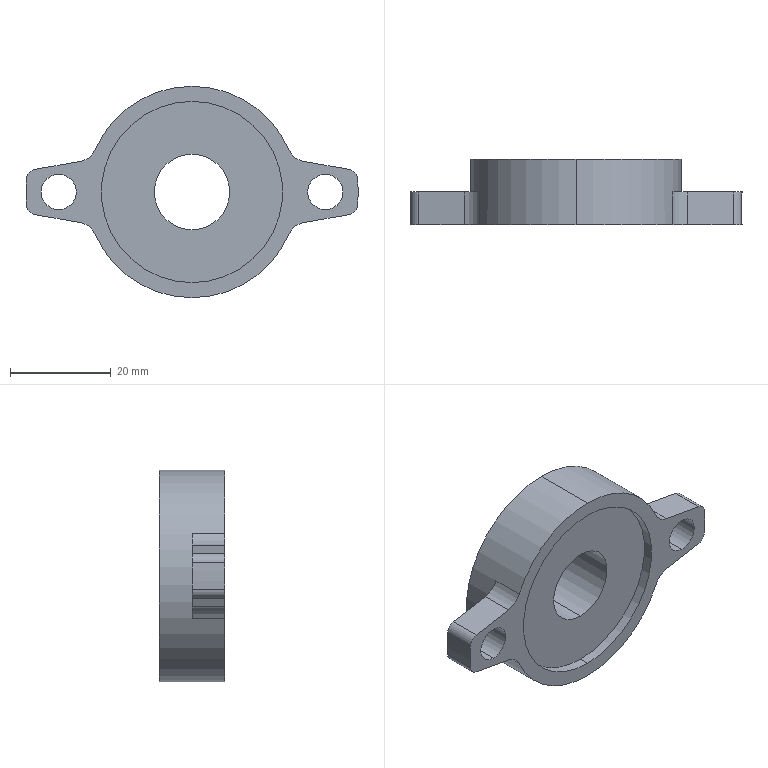Part | SolidWorks | features ICE 3, Fillet 2, Extrusion 1 | 1 solid | 29 faces | box 66 x 13 x 42 mm | volume 15219 mm3 | cylinder 20 | plane 9 | commonest cylinder face diameters 4 x4 7 x4 8 x4 15 x2 36 x2 42 x2
STEP:
#1=CARTESIAN_POINT('',(0.,2.,18.));
#2=VERTEX_POINT('',#1);
#3=CARTESIAN_POINT('',(0.,2.,-18.));
#4=VERTEX_POINT('',#3);
#5=CARTESIAN_POINT('',(0.,2.,0.));
#6=DIRECTION('',(0.,-1.,0.));
#7=DIRECTION('',(0.,0.,-1.));
#8=AXIS2_PLACEMENT_3D('',#5,#6,#7);
#9=CIRCLE('',#8,18.);
#10=EDGE_CURVE('',#2,#4,#9,.T.);
#11=ORIENTED_EDGE('',*,*,#10,.F.);
#12=CARTESIAN_POINT('',(0.,0.,18.));
#13=VERTEX_POINT('',#12);
#14=CARTESIAN_POINT('',(0.,2.,18.));
#15=DIRECTION('',(0.,-1.,0.));
#16=VECTOR('',#15,1000.);
#17=LINE('',#14,#16);
#18=EDGE_CURVE('',#2,#13,#17,.T.);
#19=ORIENTED_EDGE('',*,*,#18,.T.);
#20=CARTESIAN_POINT('',(0.,0.,-18.));
#21=VERTEX_POINT('',#20);
#22=CARTESIAN_POINT('',(0.,0.,0.));
#23=DIRECTION('',(0.,-1.,0.));
#24=DIRECTION('',(0.,0.,-1.));
#25=AXIS2_PLACEMENT_3D('',#22,#23,#24);
#26=CIRCLE('',#25,18.);
#27=EDGE_CURVE('',#13,#21,#26,.T.);
#28=ORIENTED_EDGE('',*,*,#27,.T.);
#29=CARTESIAN_POINT('',(0.,2.,-18.));
#30=DIRECTION('',(0.,-1.,0.));
#31=VECTOR('',#30,1000.);
#32=LINE('',#29,#31);
#33=EDGE_CURVE('',#4,#21,#32,.T.);
#34=ORIENTED_EDGE('',*,*,#33,.F.);
#35=EDGE_LOOP('',(#11,#19,#28,#34));
#36=FACE_OUTER_BOUND('',#35,.T.);
#37=CARTESIAN_POINT('',(0.,2.,0.));
#38=DIRECTION('',(0.,-1.,0.));
#39=DIRECTION('',(0.,0.,-1.));
#40=AXIS2_PLACEMENT_3D('',#37,#38,#39);
#41=CYLINDRICAL_SURFACE('',#40,18.);
#42=ADVANCED_FACE('',(#36),#41,.F.);
#43=CARTESIAN_POINT('',(26.5,0.,-3.5));
#44=VERTEX_POINT('',#43);
#45=CARTESIAN_POINT('',(26.5,0.,3.5));
#46=VERTEX_POINT('',#45);
#47=CARTESIAN_POINT('',(26.5,0.,0.));
#48=DIRECTION('',(0.,1.,0.));
#49=DIRECTION('',(0.,0.,1.));
#50=AXIS2_PLACEMENT_3D('',#47,#48,#49);
#51=CIRCLE('',#50,3.5);
#52=EDGE_CURVE('',#44,#46,#51,.T.);
#53=ORIENTED_EDGE('',*,*,#52,.F.);
#54=CARTESIAN_POINT('',(26.5,6.5,-3.5));
#55=VERTEX_POINT('',#54);
#56=CARTESIAN_POINT('',(26.5,0.,-3.5));
#57=DIRECTION('',(0.,1.,0.));
#58=VECTOR('',#57,1000.);
#59=LINE('',#56,#58);
#60=EDGE_CURVE('',#44,#55,#59,.T.);
#61=ORIENTED_EDGE('',*,*,#60,.T.);
#62=CARTESIAN_POINT('',(26.5,6.5,3.5));
#63=VERTEX_POINT('',#62);
#64=CARTESIAN_POINT('',(26.5,6.5,0.));
#65=DIRECTION('',(0.,1.,0.));
#66=DIRECTION('',(0.,0.,1.));
#67=AXIS2_PLACEMENT_3D('',#64,#65,#66);
#68=CIRCLE('',#67,3.5);
#69=EDGE_CURVE('',#55,#63,#68,.T.);
#70=ORIENTED_EDGE('',*,*,#69,.T.);
#71=CARTESIAN_POINT('',(26.5,0.,3.5));
#72=DIRECTION('',(0.,1.,0.));
#73=VECTOR('',#72,1000.);
#74=LINE('',#71,#73);
#75=EDGE_CURVE('',#46,#63,#74,.T.);
#76=ORIENTED_EDGE('',*,*,#75,.F.);
#77=EDGE_LOOP('',(#53,#61,#70,#76));
#78=FACE_OUTER_BOUND('',#77,.T.);
#79=CARTESIAN_POINT('',(26.5,0.,0.));
#80=DIRECTION('',(0.,1.,0.));
#81=DIRECTION('',(0.,0.,1.));
#82=AXIS2_PLACEMENT_3D('',#79,#80,#81);
#83=CYLINDRICAL_SURFACE('',#82,3.5);
#84=ADVANCED_FACE('',(#78),#83,.F.);
#85=CARTESIAN_POINT('',(-26.5,0.,-3.5));
#86=VERTEX_POINT('',#85);
#87=CARTESIAN_POINT('',(-26.5,0.,3.5));
#88=VERTEX_POINT('',#87);
#89=CARTESIAN_POINT('',(-26.5,0.,0.));
#90=DIRECTION('',(0.,1.,0.));
#91=DIRECTION('',(0.,0.,1.));
#92=AXIS2_PLACEMENT_3D('',#89,#90,#91);
#93=CIRCLE('',#92,3.5);
#94=EDGE_CURVE('',#86,#88,#93,.T.);
#95=ORIENTED_EDGE('',*,*,#94,.F.);
#96=CARTESIAN_POINT('',(-26.5,6.5,-3.5));
#97=VERTEX_POINT('',#96);
#98=CARTESIAN_POINT('',(-26.5,0.,-3.5));
#99=DIRECTION('',(0.,1.,0.));
#100=VECTOR('',#99,1000.);
#101=LINE('',#98,#100);
#102=EDGE_CURVE('',#86,#97,#101,.T.);
#103=ORIENTED_EDGE('',*,*,#102,.T.);
#104=CARTESIAN_POINT('',(-26.5,6.5,3.5));
#105=VERTEX_POINT('',#104);
#106=CARTESIAN_POINT('',(-26.5,6.5,0.));
#107=DIRECTION('',(0.,1.,0.));
#108=DIRECTION('',(0.,0.,1.));
#109=AXIS2_PLACEMENT_3D('',#106,#107,#108);
#110=CIRCLE('',#109,3.5);
#111=EDGE_CURVE('',#97,#105,#110,.T.);
#112=ORIENTED_EDGE('',*,*,#111,.T.);
#113=CARTESIAN_POINT('',(-26.5,0.,3.5));
#114=DIRECTION('',(0.,1.,0.));
#115=VECTOR('',#114,1000.);
#116=LINE('',#113,#115);
#117=EDGE_CURVE('',#88,#105,#116,.T.);
#118=ORIENTED_EDGE('',*,*,#117,.F.);
#119=EDGE_LOOP('',(#95,#103,#112,#118));
#120=FACE_OUTER_BOUND('',#119,.T.);
#121=CARTESIAN_POINT('',(-26.5,0.,0.));
#122=DIRECTION('',(0.,1.,0.));
#123=DIRECTION('',(0.,0.,1.));
#124=AXIS2_PLACEMENT_3D('',#121,#122,#123);
#125=CYLINDRICAL_SURFACE('',#124,3.5);
#126=ADVANCED_FACE('',(#120),#125,.F.);
#127=CARTESIAN_POINT('',(0.,13.,21.));
#128=VERTEX_POINT('',#127);
#129=CARTESIAN_POINT('',(0.,13.,-21.));
#130=VERTEX_POINT('',#129);
#131=CARTESIAN_POINT('',(0.,13.,0.));
#132=DIRECTION('',(0.,1.,0.));
#133=DIRECTION('',(0.,0.,1.));
#134=AXIS2_PLACEMENT_3D('',#131,#132,#133);
#135=CIRCLE('',#134,21.);
#136=EDGE_CURVE('',#128,#130,#135,.T.);
#137=ORIENTED_EDGE('',*,*,#136,.F.);
#138=CARTESIAN_POINT('',(0.,0.,21.));
#139=VERTEX_POINT('',#138);
#140=CARTESIAN_POINT('',(0.,13.,21.));
#141=DIRECTION('',(0.,-1.,0.));
#142=VECTOR('',#141,1000.);
#143=LINE('',#140,#142);
#144=EDGE_CURVE('',#128,#139,#143,.T.);
#145=ORIENTED_EDGE('',*,*,#144,.T.);
#146=CARTESIAN_POINT('',(19.238,0.,8.42));
#147=VERTEX_POINT('',#146);
#148=CARTESIAN_POINT('',(0.,0.,0.));
#149=DIRECTION('',(0.,1.,0.));
#150=DIRECTION('',(0.,0.,1.));
#151=AXIS2_PLACEMENT_3D('',#148,#149,#150);
#152=CIRCLE('',#151,21.);
#153=EDGE_CURVE('',#139,#147,#152,.T.);
#154=ORIENTED_EDGE('',*,*,#153,.T.);
#155=CARTESIAN_POINT('',(19.238,6.5,8.42));
#156=VERTEX_POINT('',#155);
#157=CARTESIAN_POINT('',(19.238,13.,8.42));
#158=DIRECTION('',(0.,1.,0.));
#159=VECTOR('',#158,1000.);
#160=LINE('',#157,#159);
#161=EDGE_CURVE('',#147,#156,#160,.T.);
#162=ORIENTED_EDGE('',*,*,#161,.T.);
#163=CARTESIAN_POINT('',(19.238,6.5,-8.42));
#164=VERTEX_POINT('',#163);
#165=CARTESIAN_POINT('',(0.,6.5,0.));
#166=DIRECTION('',(0.,1.,0.));
#167=DIRECTION('',(0.,0.,-1.));
#168=AXIS2_PLACEMENT_3D('',#165,#166,#167);
#169=CIRCLE('',#168,21.);
#170=EDGE_CURVE('',#156,#164,#169,.T.);
#171=ORIENTED_EDGE('',*,*,#170,.T.);
#172=CARTESIAN_POINT('',(19.238,0.,-8.42));
#173=VERTEX_POINT('',#172);
#174=CARTESIAN_POINT('',(19.238,13.,-8.42));
#175=DIRECTION('',(0.,-1.,0.));
#176=VECTOR('',#175,1000.);
#177=LINE('',#174,#176);
#178=EDGE_CURVE('',#164,#173,#177,.T.);
#179=ORIENTED_EDGE('',*,*,#178,.T.);
#180=CARTESIAN_POINT('',(0.,0.,-21.));
#181=VERTEX_POINT('',#180);
#182=CARTESIAN_POINT('',(0.,0.,0.));
#183=DIRECTION('',(0.,1.,0.));
#184=DIRECTION('',(0.,0.,1.));
#185=AXIS2_PLACEMENT_3D('',#182,#183,#184);
#186=CIRCLE('',#185,21.);
#187=EDGE_CURVE('',#173,#181,#186,.T.);
#188=ORIENTED_EDGE('',*,*,#187,.T.);
#189=CARTESIAN_POINT('',(0.,13.,-21.));
#190=DIRECTION('',(0.,-1.,0.));
#191=VECTOR('',#190,1000.);
#192=LINE('',#189,#191);
#193=EDGE_CURVE('',#130,#181,#192,.T.);
#194=ORIENTED_EDGE('',*,*,#193,.F.);
#195=EDGE_LOOP('',(#137,#145,#154,#162,#171,#179,#188,#194));
#196=FACE_OUTER_BOUND('',#195,.T.);
#197=CARTESIAN_POINT('',(0.,13.,0.));
#198=DIRECTION('',(0.,-1.,0.));
#199=DIRECTION('',(0.,0.,-1.));
#200=AXIS2_PLACEMENT_3D('',#197,#198,#199);
#201=CYLINDRICAL_SURFACE('',#200,21.);
#202=ADVANCED_FACE('',(#196),#201,.T.);
#203=CARTESIAN_POINT('',(0.,13.,-7.5));
#204=VERTEX_POINT('',#203);
#205=CARTESIAN_POINT('',(0.,13.,7.5));
#206=VERTEX_POINT('',#205);
#207=CARTESIAN_POINT('',(0.,13.,0.));
#208=DIRECTION('',(0.,1.,0.));
#209=DIRECTION('',(0.,0.,1.));
#210=AXIS2_PLACEMENT_3D('',#207,#208,#209);
#211=CIRCLE('',#210,7.5);
#212=EDGE_CURVE('',#204,#206,#211,.T.);
#213=ORIENTED_EDGE('',*,*,#212,.T.);
#214=CARTESIAN_POINT('',(0.,2.,7.5));
#215=VERTEX_POINT('',#214);
#216=CARTESIAN_POINT('',(0.,13.,7.5));
#217=DIRECTION('',(0.,-1.,0.));
#218=VECTOR('',#217,1000.);
#219=LINE('',#216,#218);
#220=EDGE_CURVE('',#206,#215,#219,.T.);
#221=ORIENTED_EDGE('',*,*,#220,.T.);
#222=CARTESIAN_POINT('',(0.,2.,-7.5));
#223=VERTEX_POINT('',#222);
#224=CARTESIAN_POINT('',(0.,2.,0.));
#225=DIRECTION('',(0.,-1.,0.));
#226=DIRECTION('',(0.,0.,-1.));
#227=AXIS2_PLACEMENT_3D('',#224,#225,#226);
#228=CIRCLE('',#227,7.5);
#229=EDGE_CURVE('',#215,#223,#228,.T.);
#230=ORIENTED_EDGE('',*,*,#229,.T.);
#231=CARTESIAN_POINT('',(0.,13.,-7.5));
#232=DIRECTION('',(0.,-1.,0.));
#233=VECTOR('',#232,1000.);
#234=LINE('',#231,#233);
#235=EDGE_CURVE('',#204,#223,#234,.T.);
#236=ORIENTED_EDGE('',*,*,#235,.F.);
#237=EDGE_LOOP('',(#213,#221,#230,#236));
#238=FACE_OUTER_BOUND('',#237,.T.);
#239=CARTESIAN_POINT('',(0.,13.,0.));
#240=DIRECTION('',(0.,-1.,0.));
#241=DIRECTION('',(0.,0.,-1.));
#242=AXIS2_PLACEMENT_3D('',#239,#240,#241);
#243=CYLINDRICAL_SURFACE('',#242,7.5);
#244=ADVANCED_FACE('',(#238),#243,.F.);
#245=ORIENTED_EDGE('',*,*,#220,.F.);
#246=CARTESIAN_POINT('',(0.,13.,0.));
#247=DIRECTION('',(0.,1.,0.));
#248=DIRECTION('',(0.,0.,1.));
#249=AXIS2_PLACEMENT_3D('',#246,#247,#248);
#250=CIRCLE('',#249,7.5);
#251=EDGE_CURVE('',#206,#204,#250,.T.);
#252=ORIENTED_EDGE('',*,*,#251,.T.);
#253=ORIENTED_EDGE('',*,*,#235,.T.);
#254=CARTESIAN_POINT('',(0.,2.,0.));
#255=DIRECTION('',(0.,-1.,0.));
#256=DIRECTION('',(0.,0.,-1.));
#257=AXIS2_PLACEMENT_3D('',#254,#255,#256);
#258=CIRCLE('',#257,7.5);
#259=EDGE_CURVE('',#223,#215,#258,.T.);
#260=ORIENTED_EDGE('',*,*,#259,.T.);
#261=EDGE_LOOP('',(#245,#252,#253,#260));
#262=FACE_OUTER_BOUND('',#261,.T.);
#263=CARTESIAN_POINT('',(0.,13.,0.));
#264=DIRECTION('',(0.,-1.,0.));
#265=DIRECTION('',(0.,0.,-1.));
#266=AXIS2_PLACEMENT_3D('',#263,#264,#265);
#267=CYLINDRICAL_SURFACE('',#266,7.5);
#268=ADVANCED_FACE('',(#262),#267,.F.);
#269=CARTESIAN_POINT('',(0.,13.,0.));
#270=DIRECTION('',(0.,1.,0.));
#271=DIRECTION('',(0.,0.,1.));
#272=AXIS2_PLACEMENT_3D('',#269,#270,#271);
#273=CIRCLE('',#272,21.);
#274=EDGE_CURVE('',#130,#128,#273,.T.);
#275=ORIENTED_EDGE('',*,*,#274,.T.);
#276=ORIENTED_EDGE('',*,*,#136,.T.);
#277=EDGE_LOOP('',(#275,#276));
#278=FACE_OUTER_BOUND('',#277,.T.);
#279=ORIENTED_EDGE('',*,*,#212,.F.);
#280=ORIENTED_EDGE('',*,*,#251,.F.);
#281=EDGE_LOOP('',(#279,#280));
#282=FACE_BOUND('',#281,.T.);
#283=CARTESIAN_POINT('',(0.,13.,0.));
#284=DIRECTION('',(0.,1.,0.));
#285=DIRECTION('',(0.,0.,1.));
#286=AXIS2_PLACEMENT_3D('',#283,#284,#285);
#287=PLANE('',#286);
#288=ADVANCED_FACE('',(#278,#282),#287,.T.);
#289=CARTESIAN_POINT('',(0.,0.,0.));
#290=DIRECTION('',(0.,-1.,0.));
#291=DIRECTION('',(0.,0.,-1.));
#292=AXIS2_PLACEMENT_3D('',#289,#290,#291);
#293=CIRCLE('',#292,18.);
#294=EDGE_CURVE('',#21,#13,#293,.T.);
#295=ORIENTED_EDGE('',*,*,#294,.F.);
#296=ORIENTED_EDGE('',*,*,#27,.F.);
#297=EDGE_LOOP('',(#295,#296));
#298=FACE_BOUND('',#297,.T.);
#299=CARTESIAN_POINT('',(26.5,0.,0.));
#300=DIRECTION('',(0.,1.,0.));
#301=DIRECTION('',(0.,0.,1.));
#302=AXIS2_PLACEMENT_3D('',#299,#300,#301);
#303=CIRCLE('',#302,3.5);
#304=EDGE_CURVE('',#46,#44,#303,.T.);
#305=ORIENTED_EDGE('',*,*,#304,.T.);
#306=ORIENTED_EDGE('',*,*,#52,.T.);
#307=EDGE_LOOP('',(#305,#306));
#308=FACE_BOUND('',#307,.T.);
#309=CARTESIAN_POINT('',(-26.5,0.,0.));
#310=DIRECTION('',(0.,1.,0.));
#311=DIRECTION('',(0.,0.,1.));
#312=AXIS2_PLACEMENT_3D('',#309,#310,#311);
#313=CIRCLE('',#312,3.5);
#314=EDGE_CURVE('',#88,#86,#313,.T.);
#315=ORIENTED_EDGE('',*,*,#314,.T.);
#316=ORIENTED_EDGE('',*,*,#94,.T.);
#317=EDGE_LOOP('',(#315,#316));
#318=FACE_BOUND('',#317,.T.);
#319=CARTESIAN_POINT('',(32.891,0.,-2.684));
#320=VERTEX_POINT('',#319);
#321=CARTESIAN_POINT('',(32.891,0.,2.684));
#322=VERTEX_POINT('',#321);
#323=CARTESIAN_POINT('',(0.,0.,0.));
#324=DIRECTION('',(0.,-1.,0.));
#325=DIRECTION('',(0.,0.,-1.));
#326=AXIS2_PLACEMENT_3D('',#323,#324,#325);
#327=CIRCLE('',#326,33.);
#328=EDGE_CURVE('',#320,#322,#327,.T.);
#329=ORIENTED_EDGE('',*,*,#328,.T.);
#330=CARTESIAN_POINT('',(31.245,0.,4.491));
#331=VERTEX_POINT('',#330);
#332=CARTESIAN_POINT('',(30.897,0.,2.521));
#333=DIRECTION('',(0.,-1.,0.));
#334=DIRECTION('',(0.,0.,1.));
#335=AXIS2_PLACEMENT_3D('',#332,#333,#334);
#336=CIRCLE('',#335,2.);
#337=EDGE_CURVE('',#322,#331,#336,.T.);
#338=ORIENTED_EDGE('',*,*,#337,.T.);
#339=CARTESIAN_POINT('',(22.208,0.,6.084));
#340=VERTEX_POINT('',#339);
#341=CARTESIAN_POINT('',(32.728,0.,4.229));
#342=DIRECTION('',(-0.9848,0.,0.1736));
#343=VECTOR('',#342,1000.);
#344=LINE('',#341,#343);
#345=EDGE_CURVE('',#331,#340,#344,.T.);
#346=ORIENTED_EDGE('',*,*,#345,.T.);
#347=CARTESIAN_POINT('',(22.903,0.,10.023));
#348=DIRECTION('',(0.,1.,0.));
#349=DIRECTION('',(0.,0.,1.));
#350=AXIS2_PLACEMENT_3D('',#347,#348,#349);
#351=CIRCLE('',#350,4.);
#352=EDGE_CURVE('',#340,#147,#351,.T.);
#353=ORIENTED_EDGE('',*,*,#352,.T.);
#354=ORIENTED_EDGE('',*,*,#153,.F.);
#355=CARTESIAN_POINT('',(-19.238,0.,8.42));
#356=VERTEX_POINT('',#355);
#357=CARTESIAN_POINT('',(0.,0.,0.));
#358=DIRECTION('',(0.,1.,0.));
#359=DIRECTION('',(0.,0.,1.));
#360=AXIS2_PLACEMENT_3D('',#357,#358,#359);
#361=CIRCLE('',#360,21.);
#362=EDGE_CURVE('',#356,#139,#361,.T.);
#363=ORIENTED_EDGE('',*,*,#362,.F.);
#364=CARTESIAN_POINT('',(-22.208,0.,6.084));
#365=VERTEX_POINT('',#364);
#366=CARTESIAN_POINT('',(-22.903,0.,10.023));
#367=DIRECTION('',(0.,1.,0.));
#368=DIRECTION('',(0.,0.,1.));
#369=AXIS2_PLACEMENT_3D('',#366,#367,#368);
#370=CIRCLE('',#369,4.);
#371=EDGE_CURVE('',#356,#365,#370,.T.);
#372=ORIENTED_EDGE('',*,*,#371,.T.);
#373=CARTESIAN_POINT('',(-31.245,0.,4.491));
#374=VERTEX_POINT('',#373);
#375=CARTESIAN_POINT('',(-32.728,0.,4.229));
#376=DIRECTION('',(-0.9848,0.,-0.1736));
#377=VECTOR('',#376,1000.);
#378=LINE('',#375,#377);
#379=EDGE_CURVE('',#365,#374,#378,.T.);
#380=ORIENTED_EDGE('',*,*,#379,.T.);
#381=CARTESIAN_POINT('',(-32.891,0.,2.684));
#382=VERTEX_POINT('',#381);
#383=CARTESIAN_POINT('',(-30.897,0.,2.521));
#384=DIRECTION('',(0.,-1.,0.));
#385=DIRECTION('',(0.,0.,1.));
#386=AXIS2_PLACEMENT_3D('',#383,#384,#385);
#387=CIRCLE('',#386,2.);
#388=EDGE_CURVE('',#374,#382,#387,.T.);
#389=ORIENTED_EDGE('',*,*,#388,.T.);
#390=CARTESIAN_POINT('',(-32.891,0.,-2.684));
#391=VERTEX_POINT('',#390);
#392=CARTESIAN_POINT('',(0.,0.,0.));
#393=DIRECTION('',(0.,-1.,0.));
#394=DIRECTION('',(0.,0.,-1.));
#395=AXIS2_PLACEMENT_3D('',#392,#393,#394);
#396=CIRCLE('',#395,33.);
#397=EDGE_CURVE('',#382,#391,#396,.T.);
#398=ORIENTED_EDGE('',*,*,#397,.T.);
#399=CARTESIAN_POINT('',(-31.245,0.,-4.491));
#400=VERTEX_POINT('',#399);
#401=CARTESIAN_POINT('',(-30.897,0.,-2.521));
#402=DIRECTION('',(0.,-1.,0.));
#403=DIRECTION('',(0.,0.,1.));
#404=AXIS2_PLACEMENT_3D('',#401,#402,#403);
#405=CIRCLE('',#404,2.);
#406=EDGE_CURVE('',#391,#400,#405,.T.);
#407=ORIENTED_EDGE('',*,*,#406,.T.);
#408=CARTESIAN_POINT('',(-22.208,0.,-6.084));
#409=VERTEX_POINT('',#408);
#410=CARTESIAN_POINT('',(-32.728,0.,-4.229));
#411=DIRECTION('',(0.9848,0.,-0.1736));
#412=VECTOR('',#411,1000.);
#413=LINE('',#410,#412);
#414=EDGE_CURVE('',#400,#409,#413,.T.);
#415=ORIENTED_EDGE('',*,*,#414,.T.);
#416=CARTESIAN_POINT('',(-19.238,0.,-8.42));
#417=VERTEX_POINT('',#416);
#418=CARTESIAN_POINT('',(-22.903,0.,-10.023));
#419=DIRECTION('',(0.,1.,0.));
#420=DIRECTION('',(0.,0.,1.));
#421=AXIS2_PLACEMENT_3D('',#418,#419,#420);
#422=CIRCLE('',#421,4.);
#423=EDGE_CURVE('',#409,#417,#422,.T.);
#424=ORIENTED_EDGE('',*,*,#423,.T.);
#425=CARTESIAN_POINT('',(0.,0.,0.));
#426=DIRECTION('',(0.,1.,0.));
#427=DIRECTION('',(0.,0.,1.));
#428=AXIS2_PLACEMENT_3D('',#425,#426,#427);
#429=CIRCLE('',#428,21.);
#430=EDGE_CURVE('',#181,#417,#429,.T.);
#431=ORIENTED_EDGE('',*,*,#430,.F.);
#432=ORIENTED_EDGE('',*,*,#187,.F.);
#433=CARTESIAN_POINT('',(22.208,0.,-6.084));
#434=VERTEX_POINT('',#433);
#435=CARTESIAN_POINT('',(22.903,0.,-10.023));
#436=DIRECTION('',(0.,1.,0.));
#437=DIRECTION('',(0.,0.,1.));
#438=AXIS2_PLACEMENT_3D('',#435,#436,#437);
#439=CIRCLE('',#438,4.);
#440=EDGE_CURVE('',#173,#434,#439,.T.);
#441=ORIENTED_EDGE('',*,*,#440,.T.);
#442=CARTESIAN_POINT('',(31.245,0.,-4.491));
#443=VERTEX_POINT('',#442);
#444=CARTESIAN_POINT('',(32.728,0.,-4.229));
#445=DIRECTION('',(0.9848,0.,0.1736));
#446=VECTOR('',#445,1000.);
#447=LINE('',#444,#446);
#448=EDGE_CURVE('',#434,#443,#447,.T.);
#449=ORIENTED_EDGE('',*,*,#448,.T.);
#450=CARTESIAN_POINT('',(30.897,0.,-2.521));
#451=DIRECTION('',(0.,-1.,0.));
#452=DIRECTION('',(0.,0.,1.));
#453=AXIS2_PLACEMENT_3D('',#450,#451,#452);
#454=CIRCLE('',#453,2.);
#455=EDGE_CURVE('',#443,#320,#454,.T.);
#456=ORIENTED_EDGE('',*,*,#455,.T.);
#457=EDGE_LOOP('',(#329,#338,#346,#353,#354,#363,#372,#380,#389,#398,#407,#415,#424,#431,#432,#441,#449,#456));
#458=FACE_OUTER_BOUND('',#457,.T.);
#459=CARTESIAN_POINT('',(0.,0.,0.));
#460=DIRECTION('',(0.,1.,0.));
#461=DIRECTION('',(0.,0.,1.));
#462=AXIS2_PLACEMENT_3D('',#459,#460,#461);
#463=PLANE('',#462);
#464=ADVANCED_FACE('',(#298,#308,#318,#458),#463,.F.);
#465=ORIENTED_EDGE('',*,*,#144,.F.);
#466=ORIENTED_EDGE('',*,*,#274,.F.);
#467=ORIENTED_EDGE('',*,*,#193,.T.);
#468=ORIENTED_EDGE('',*,*,#430,.T.);
#469=CARTESIAN_POINT('',(-19.238,6.5,-8.42));
#470=VERTEX_POINT('',#469);
#471=CARTESIAN_POINT('',(-19.238,13.,-8.42));
#472=DIRECTION('',(0.,1.,0.));
#473=VECTOR('',#472,1000.);
#474=LINE('',#471,#473);
#475=EDGE_CURVE('',#417,#470,#474,.T.);
#476=ORIENTED_EDGE('',*,*,#475,.T.);
#477=CARTESIAN_POINT('',(-19.238,6.5,8.42));
#478=VERTEX_POINT('',#477);
#479=CARTESIAN_POINT('',(0.,6.5,0.));
#480=DIRECTION('',(0.,1.,0.));
#481=DIRECTION('',(0.,0.,-1.));
#482=AXIS2_PLACEMENT_3D('',#479,#480,#481);
#483=CIRCLE('',#482,21.);
#484=EDGE_CURVE('',#470,#478,#483,.T.);
#485=ORIENTED_EDGE('',*,*,#484,.T.);
#486=CARTESIAN_POINT('',(-19.238,13.,8.42));
#487=DIRECTION('',(0.,-1.,0.));
#488=VECTOR('',#487,1000.);
#489=LINE('',#486,#488);
#490=EDGE_CURVE('',#478,#356,#489,.T.);
#491=ORIENTED_EDGE('',*,*,#490,.T.);
#492=ORIENTED_EDGE('',*,*,#362,.T.);
#493=EDGE_LOOP('',(#465,#466,#467,#468,#476,#485,#491,#492));
#494=FACE_OUTER_BOUND('',#493,.T.);
#495=CARTESIAN_POINT('',(0.,13.,0.));
#496=DIRECTION('',(0.,-1.,0.));
#497=DIRECTION('',(0.,0.,-1.));
#498=AXIS2_PLACEMENT_3D('',#495,#496,#497);
#499=CYLINDRICAL_SURFACE('',#498,21.);
#500=ADVANCED_FACE('',(#494),#499,.T.);
#501=CARTESIAN_POINT('',(32.891,6.5,-2.684));
#502=VERTEX_POINT('',#501);
#503=CARTESIAN_POINT('',(32.891,6.5,2.684));
#504=VERTEX_POINT('',#503);
#505=CARTESIAN_POINT('',(0.,6.5,0.));
#506=DIRECTION('',(0.,-1.,0.));
#507=DIRECTION('',(0.,0.,-1.));
#508=AXIS2_PLACEMENT_3D('',#505,#506,#507);
#509=CIRCLE('',#508,33.);
#510=EDGE_CURVE('',#502,#504,#509,.T.);
#511=ORIENTED_EDGE('',*,*,#510,.T.);
#512=CARTESIAN_POINT('',(32.891,6.5,2.684));
#513=DIRECTION('',(0.,-1.,0.));
#514=VECTOR('',#513,1000.);
#515=LINE('',#512,#514);
#516=EDGE_CURVE('',#504,#322,#515,.T.);
#517=ORIENTED_EDGE('',*,*,#516,.T.);
#518=ORIENTED_EDGE('',*,*,#328,.F.);
#519=CARTESIAN_POINT('',(32.891,6.5,-2.684));
#520=DIRECTION('',(0.,1.,0.));
#521=VECTOR('',#520,1000.);
#522=LINE('',#519,#521);
#523=EDGE_CURVE('',#320,#502,#522,.T.);
#524=ORIENTED_EDGE('',*,*,#523,.T.);
#525=EDGE_LOOP('',(#511,#517,#518,#524));
#526=FACE_OUTER_BOUND('',#525,.T.);
#527=CARTESIAN_POINT('',(0.,6.5,0.));
#528=DIRECTION('',(0.,-1.,0.));
#529=DIRECTION('',(0.,0.,-1.));
#530=AXIS2_PLACEMENT_3D('',#527,#528,#529);
#531=CYLINDRICAL_SURFACE('',#530,33.);
#532=ADVANCED_FACE('',(#526),#531,.T.);
#533=CARTESIAN_POINT('',(22.208,6.5,-6.084));
#534=VERTEX_POINT('',#533);
#535=CARTESIAN_POINT('',(31.245,6.5,-4.491));
#536=VERTEX_POINT('',#535);
#537=CARTESIAN_POINT('',(32.728,6.5,-4.229));
#538=DIRECTION('',(0.9848,0.,0.1736));
#539=VECTOR('',#538,1000.);
#540=LINE('',#537,#539);
#541=EDGE_CURVE('',#534,#536,#540,.T.);
#542=ORIENTED_EDGE('',*,*,#541,.T.);
#543=CARTESIAN_POINT('',(31.245,6.5,-4.491));
#544=DIRECTION('',(0.,-1.,0.));
#545=VECTOR('',#544,1000.);
#546=LINE('',#543,#545);
#547=EDGE_CURVE('',#536,#443,#546,.T.);
#548=ORIENTED_EDGE('',*,*,#547,.T.);
#549=ORIENTED_EDGE('',*,*,#448,.F.);
#550=CARTESIAN_POINT('',(22.208,6.5,-6.084));
#551=DIRECTION('',(0.,1.,0.));
#552=VECTOR('',#551,1000.);
#553=LINE('',#550,#552);
#554=EDGE_CURVE('',#434,#534,#553,.T.);
#555=ORIENTED_EDGE('',*,*,#554,.T.);
#556=EDGE_LOOP('',(#542,#548,#549,#555));
#557=FACE_OUTER_BOUND('',#556,.T.);
#558=CARTESIAN_POINT('',(32.728,6.5,-4.229));
#559=DIRECTION('',(0.1736,0.,-0.9848));
#560=DIRECTION('',(-0.9848,0.,-0.1736));
#561=AXIS2_PLACEMENT_3D('',#558,#559,#560);
#562=PLANE('',#561);
#563=ADVANCED_FACE('',(#557),#562,.T.);
#564=ORIENTED_EDGE('',*,*,#345,.F.);
#565=CARTESIAN_POINT('',(31.245,6.5,4.491));
#566=VERTEX_POINT('',#565);
#567=CARTESIAN_POINT('',(31.245,6.5,4.491));
#568=DIRECTION('',(0.,1.,0.));
#569=VECTOR('',#568,1000.);
#570=LINE('',#567,#569);
#571=EDGE_CURVE('',#331,#566,#570,.T.);
#572=ORIENTED_EDGE('',*,*,#571,.T.);
#573=CARTESIAN_POINT('',(22.208,6.5,6.084));
#574=VERTEX_POINT('',#573);
#575=CARTESIAN_POINT('',(32.728,6.5,4.229));
#576=DIRECTION('',(-0.9848,0.,0.1736));
#577=VECTOR('',#576,1000.);
#578=LINE('',#575,#577);
#579=EDGE_CURVE('',#566,#574,#578,.T.);
#580=ORIENTED_EDGE('',*,*,#579,.T.);
#581=CARTESIAN_POINT('',(22.208,6.5,6.084));
#582=DIRECTION('',(0.,-1.,0.));
#583=VECTOR('',#582,1000.);
#584=LINE('',#581,#583);
#585=EDGE_CURVE('',#574,#340,#584,.T.);
#586=ORIENTED_EDGE('',*,*,#585,.T.);
#587=EDGE_LOOP('',(#564,#572,#580,#586));
#588=FACE_OUTER_BOUND('',#587,.T.);
#589=CARTESIAN_POINT('',(32.728,6.5,4.229));
#590=DIRECTION('',(0.1736,0.,0.9848));
#591=DIRECTION('',(0.9848,0.,-0.1736));
#592=AXIS2_PLACEMENT_3D('',#589,#590,#591);
#593=PLANE('',#592);
#594=ADVANCED_FACE('',(#588),#593,.T.);
#595=CARTESIAN_POINT('',(26.5,6.5,0.));
#596=DIRECTION('',(0.,1.,0.));
#597=DIRECTION('',(0.,0.,1.));
#598=AXIS2_PLACEMENT_3D('',#595,#596,#597);
#599=CIRCLE('',#598,3.5);
#600=EDGE_CURVE('',#63,#55,#599,.T.);
#601=ORIENTED_EDGE('',*,*,#600,.F.);
#602=ORIENTED_EDGE('',*,*,#69,.F.);
#603=EDGE_LOOP('',(#601,#602));
#604=FACE_BOUND('',#603,.T.);
#605=ORIENTED_EDGE('',*,*,#579,.F.);
#606=CARTESIAN_POINT('',(30.897,6.5,2.521));
#607=DIRECTION('',(0.,1.,0.));
#608=DIRECTION('',(0.,0.,-1.));
#609=AXIS2_PLACEMENT_3D('',#606,#607,#608);
#610=CIRCLE('',#609,2.);
#611=EDGE_CURVE('',#566,#504,#610,.T.);
#612=ORIENTED_EDGE('',*,*,#611,.T.);
#613=ORIENTED_EDGE('',*,*,#510,.F.);
#614=CARTESIAN_POINT('',(30.897,6.5,-2.521));
#615=DIRECTION('',(0.,1.,0.));
#616=DIRECTION('',(0.,0.,-1.));
#617=AXIS2_PLACEMENT_3D('',#614,#615,#616);
#618=CIRCLE('',#617,2.);
#619=EDGE_CURVE('',#502,#536,#618,.T.);
#620=ORIENTED_EDGE('',*,*,#619,.T.);
#621=ORIENTED_EDGE('',*,*,#541,.F.);
#622=CARTESIAN_POINT('',(22.903,6.5,-10.023));
#623=DIRECTION('',(0.,-1.,0.));
#624=DIRECTION('',(0.,0.,-1.));
#625=AXIS2_PLACEMENT_3D('',#622,#623,#624);
#626=CIRCLE('',#625,4.);
#627=EDGE_CURVE('',#534,#164,#626,.T.);
#628=ORIENTED_EDGE('',*,*,#627,.T.);
#629=ORIENTED_EDGE('',*,*,#170,.F.);
#630=CARTESIAN_POINT('',(22.903,6.5,10.023));
#631=DIRECTION('',(0.,-1.,0.));
#632=DIRECTION('',(0.,0.,-1.));
#633=AXIS2_PLACEMENT_3D('',#630,#631,#632);
#634=CIRCLE('',#633,4.);
#635=EDGE_CURVE('',#156,#574,#634,.T.);
#636=ORIENTED_EDGE('',*,*,#635,.T.);
#637=EDGE_LOOP('',(#605,#612,#613,#620,#621,#628,#629,#636));
#638=FACE_OUTER_BOUND('',#637,.T.);
#639=CARTESIAN_POINT('',(0.,6.5,0.));
#640=DIRECTION('',(0.,-1.,0.));
#641=DIRECTION('',(0.,0.,-1.));
#642=AXIS2_PLACEMENT_3D('',#639,#640,#641);
#643=PLANE('',#642);
#644=ADVANCED_FACE('',(#604,#638),#643,.F.);
#645=CARTESIAN_POINT('',(-32.891,6.5,2.684));
#646=VERTEX_POINT('',#645);
#647=CARTESIAN_POINT('',(-32.891,6.5,-2.684));
#648=VERTEX_POINT('',#647);
#649=CARTESIAN_POINT('',(0.,6.5,0.));
#650=DIRECTION('',(0.,-1.,0.));
#651=DIRECTION('',(0.,0.,-1.));
#652=AXIS2_PLACEMENT_3D('',#649,#650,#651);
#653=CIRCLE('',#652,33.);
#654=EDGE_CURVE('',#646,#648,#653,.T.);
#655=ORIENTED_EDGE('',*,*,#654,.T.);
#656=CARTESIAN_POINT('',(-32.891,6.5,-2.684));
#657=DIRECTION('',(0.,-1.,0.));
#658=VECTOR('',#657,1000.);
#659=LINE('',#656,#658);
#660=EDGE_CURVE('',#648,#391,#659,.T.);
#661=ORIENTED_EDGE('',*,*,#660,.T.);
#662=ORIENTED_EDGE('',*,*,#397,.F.);
#663=CARTESIAN_POINT('',(-32.891,6.5,2.684));
#664=DIRECTION('',(0.,1.,0.));
#665=VECTOR('',#664,1000.);
#666=LINE('',#663,#665);
#667=EDGE_CURVE('',#382,#646,#666,.T.);
#668=ORIENTED_EDGE('',*,*,#667,.T.);
#669=EDGE_LOOP('',(#655,#661,#662,#668));
#670=FACE_OUTER_BOUND('',#669,.T.);
#671=CARTESIAN_POINT('',(0.,6.5,0.));
#672=DIRECTION('',(0.,-1.,0.));
#673=DIRECTION('',(0.,0.,-1.));
#674=AXIS2_PLACEMENT_3D('',#671,#672,#673);
#675=CYLINDRICAL_SURFACE('',#674,33.);
#676=ADVANCED_FACE('',(#670),#675,.T.);
#677=CARTESIAN_POINT('',(-22.208,6.5,6.084));
#678=VERTEX_POINT('',#677);
#679=CARTESIAN_POINT('',(-31.245,6.5,4.491));
#680=VERTEX_POINT('',#679);
#681=CARTESIAN_POINT('',(-32.728,6.5,4.229));
#682=DIRECTION('',(-0.9848,0.,-0.1736));
#683=VECTOR('',#682,1000.);
#684=LINE('',#681,#683);
#685=EDGE_CURVE('',#678,#680,#684,.T.);
#686=ORIENTED_EDGE('',*,*,#685,.T.);
#687=CARTESIAN_POINT('',(-31.245,6.5,4.491));
#688=DIRECTION('',(0.,-1.,0.));
#689=VECTOR('',#688,1000.);
#690=LINE('',#687,#689);
#691=EDGE_CURVE('',#680,#374,#690,.T.);
#692=ORIENTED_EDGE('',*,*,#691,.T.);
#693=ORIENTED_EDGE('',*,*,#379,.F.);
#694=CARTESIAN_POINT('',(-22.208,6.5,6.084));
#695=DIRECTION('',(0.,1.,0.));
#696=VECTOR('',#695,1000.);
#697=LINE('',#694,#696);
#698=EDGE_CURVE('',#365,#678,#697,.T.);
#699=ORIENTED_EDGE('',*,*,#698,.T.);
#700=EDGE_LOOP('',(#686,#692,#693,#699));
#701=FACE_OUTER_BOUND('',#700,.T.);
#702=CARTESIAN_POINT('',(-32.728,6.5,4.229));
#703=DIRECTION('',(-0.1736,0.,0.9848));
#704=DIRECTION('',(0.9848,0.,0.1736));
#705=AXIS2_PLACEMENT_3D('',#702,#703,#704);
#706=PLANE('',#705);
#707=ADVANCED_FACE('',(#701),#706,.T.);
#708=ORIENTED_EDGE('',*,*,#414,.F.);
#709=CARTESIAN_POINT('',(-31.245,6.5,-4.491));
#710=VERTEX_POINT('',#709);
#711=CARTESIAN_POINT('',(-31.245,6.5,-4.491));
#712=DIRECTION('',(0.,1.,0.));
#713=VECTOR('',#712,1000.);
#714=LINE('',#711,#713);
#715=EDGE_CURVE('',#400,#710,#714,.T.);
#716=ORIENTED_EDGE('',*,*,#715,.T.);
#717=CARTESIAN_POINT('',(-22.208,6.5,-6.084));
#718=VERTEX_POINT('',#717);
#719=CARTESIAN_POINT('',(-32.728,6.5,-4.229));
#720=DIRECTION('',(0.9848,0.,-0.1736));
#721=VECTOR('',#720,1000.);
#722=LINE('',#719,#721);
#723=EDGE_CURVE('',#710,#718,#722,.T.);
#724=ORIENTED_EDGE('',*,*,#723,.T.);
#725=CARTESIAN_POINT('',(-22.208,6.5,-6.084));
#726=DIRECTION('',(0.,-1.,0.));
#727=VECTOR('',#726,1000.);
#728=LINE('',#725,#727);
#729=EDGE_CURVE('',#718,#409,#728,.T.);
#730=ORIENTED_EDGE('',*,*,#729,.T.);
#731=EDGE_LOOP('',(#708,#716,#724,#730));
#732=FACE_OUTER_BOUND('',#731,.T.);
#733=CARTESIAN_POINT('',(-32.728,6.5,-4.229));
#734=DIRECTION('',(-0.1736,0.,-0.9848));
#735=DIRECTION('',(-0.9848,0.,0.1736));
#736=AXIS2_PLACEMENT_3D('',#733,#734,#735);
#737=PLANE('',#736);
#738=ADVANCED_FACE('',(#732),#737,.T.);
#739=CARTESIAN_POINT('',(-26.5,6.5,0.));
#740=DIRECTION('',(0.,1.,0.));
#741=DIRECTION('',(0.,0.,1.));
#742=AXIS2_PLACEMENT_3D('',#739,#740,#741);
#743=CIRCLE('',#742,3.5);
#744=EDGE_CURVE('',#105,#97,#743,.T.);
#745=ORIENTED_EDGE('',*,*,#744,.F.);
#746=ORIENTED_EDGE('',*,*,#111,.F.);
#747=EDGE_LOOP('',(#745,#746));
#748=FACE_BOUND('',#747,.T.);
#749=ORIENTED_EDGE('',*,*,#723,.F.);
#750=CARTESIAN_POINT('',(-30.897,6.5,-2.521));
#751=DIRECTION('',(0.,1.,0.));
#752=DIRECTION('',(0.,0.,-1.));
#753=AXIS2_PLACEMENT_3D('',#750,#751,#752);
#754=CIRCLE('',#753,2.);
#755=EDGE_CURVE('',#710,#648,#754,.T.);
#756=ORIENTED_EDGE('',*,*,#755,.T.);
#757=ORIENTED_EDGE('',*,*,#654,.F.);
#758=CARTESIAN_POINT('',(-30.897,6.5,2.521));
#759=DIRECTION('',(0.,1.,0.));
#760=DIRECTION('',(0.,0.,-1.));
#761=AXIS2_PLACEMENT_3D('',#758,#759,#760);
#762=CIRCLE('',#761,2.);
#763=EDGE_CURVE('',#646,#680,#762,.T.);
#764=ORIENTED_EDGE('',*,*,#763,.T.);
#765=ORIENTED_EDGE('',*,*,#685,.F.);
#766=CARTESIAN_POINT('',(-22.903,6.5,10.023));
#767=DIRECTION('',(0.,-1.,0.));
#768=DIRECTION('',(0.,0.,-1.));
#769=AXIS2_PLACEMENT_3D('',#766,#767,#768);
#770=CIRCLE('',#769,4.);
#771=EDGE_CURVE('',#678,#478,#770,.T.);
#772=ORIENTED_EDGE('',*,*,#771,.T.);
#773=ORIENTED_EDGE('',*,*,#484,.F.);
#774=CARTESIAN_POINT('',(-22.903,6.5,-10.023));
#775=DIRECTION('',(0.,-1.,0.));
#776=DIRECTION('',(0.,0.,-1.));
#777=AXIS2_PLACEMENT_3D('',#774,#775,#776);
#778=CIRCLE('',#777,4.);
#779=EDGE_CURVE('',#470,#718,#778,.T.);
#780=ORIENTED_EDGE('',*,*,#779,.T.);
#781=EDGE_LOOP('',(#749,#756,#757,#764,#765,#772,#773,#780));
#782=FACE_OUTER_BOUND('',#781,.T.);
#783=CARTESIAN_POINT('',(0.,6.5,0.));
#784=DIRECTION('',(0.,-1.,0.));
#785=DIRECTION('',(0.,0.,-1.));
#786=AXIS2_PLACEMENT_3D('',#783,#784,#785);
#787=PLANE('',#786);
#788=ADVANCED_FACE('',(#748,#782),#787,.F.);
#789=ORIENTED_EDGE('',*,*,#771,.F.);
#790=ORIENTED_EDGE('',*,*,#698,.F.);
#791=ORIENTED_EDGE('',*,*,#371,.F.);
#792=ORIENTED_EDGE('',*,*,#490,.F.);
#793=EDGE_LOOP('',(#789,#790,#791,#792));
#794=FACE_OUTER_BOUND('',#793,.T.);
#795=CARTESIAN_POINT('',(-22.903,13.,10.023));
#796=DIRECTION('',(0.,-1.,0.));
#797=DIRECTION('',(0.,0.,-1.));
#798=AXIS2_PLACEMENT_3D('',#795,#796,#797);
#799=CYLINDRICAL_SURFACE('',#798,4.);
#800=ADVANCED_FACE('',(#794),#799,.F.);
#801=ORIENTED_EDGE('',*,*,#779,.F.);
#802=ORIENTED_EDGE('',*,*,#475,.F.);
#803=ORIENTED_EDGE('',*,*,#423,.F.);
#804=ORIENTED_EDGE('',*,*,#729,.F.);
#805=EDGE_LOOP('',(#801,#802,#803,#804));
#806=FACE_OUTER_BOUND('',#805,.T.);
#807=CARTESIAN_POINT('',(-22.903,13.,-10.023));
#808=DIRECTION('',(0.,-1.,0.));
#809=DIRECTION('',(0.,0.,-1.));
#810=AXIS2_PLACEMENT_3D('',#807,#808,#809);
#811=CYLINDRICAL_SURFACE('',#810,4.);
#812=ADVANCED_FACE('',(#806),#811,.F.);
#813=ORIENTED_EDGE('',*,*,#627,.F.);
#814=ORIENTED_EDGE('',*,*,#554,.F.);
#815=ORIENTED_EDGE('',*,*,#440,.F.);
#816=ORIENTED_EDGE('',*,*,#178,.F.);
#817=EDGE_LOOP('',(#813,#814,#815,#816));
#818=FACE_OUTER_BOUND('',#817,.T.);
#819=CARTESIAN_POINT('',(22.903,13.,-10.023));
#820=DIRECTION('',(0.,-1.,0.));
#821=DIRECTION('',(0.,0.,-1.));
#822=AXIS2_PLACEMENT_3D('',#819,#820,#821);
#823=CYLINDRICAL_SURFACE('',#822,4.);
#824=ADVANCED_FACE('',(#818),#823,.F.);
#825=ORIENTED_EDGE('',*,*,#635,.F.);
#826=ORIENTED_EDGE('',*,*,#161,.F.);
#827=ORIENTED_EDGE('',*,*,#352,.F.);
#828=ORIENTED_EDGE('',*,*,#585,.F.);
#829=EDGE_LOOP('',(#825,#826,#827,#828));
#830=FACE_OUTER_BOUND('',#829,.T.);
#831=CARTESIAN_POINT('',(22.903,13.,10.023));
#832=DIRECTION('',(0.,-1.,0.));
#833=DIRECTION('',(0.,0.,-1.));
#834=AXIS2_PLACEMENT_3D('',#831,#832,#833);
#835=CYLINDRICAL_SURFACE('',#834,4.);
#836=ADVANCED_FACE('',(#830),#835,.F.);
#837=ORIENTED_EDGE('',*,*,#611,.F.);
#838=ORIENTED_EDGE('',*,*,#571,.F.);
#839=ORIENTED_EDGE('',*,*,#337,.F.);
#840=ORIENTED_EDGE('',*,*,#516,.F.);
#841=EDGE_LOOP('',(#837,#838,#839,#840));
#842=FACE_OUTER_BOUND('',#841,.T.);
#843=CARTESIAN_POINT('',(30.897,6.5,2.521));
#844=DIRECTION('',(0.,-1.,0.));
#845=DIRECTION('',(0.,0.,-1.));
#846=AXIS2_PLACEMENT_3D('',#843,#844,#845);
#847=CYLINDRICAL_SURFACE('',#846,2.);
#848=ADVANCED_FACE('',(#842),#847,.T.);
#849=ORIENTED_EDGE('',*,*,#619,.F.);
#850=ORIENTED_EDGE('',*,*,#523,.F.);
#851=ORIENTED_EDGE('',*,*,#455,.F.);
#852=ORIENTED_EDGE('',*,*,#547,.F.);
#853=EDGE_LOOP('',(#849,#850,#851,#852));
#854=FACE_OUTER_BOUND('',#853,.T.);
#855=CARTESIAN_POINT('',(30.897,6.5,-2.521));
#856=DIRECTION('',(0.,-1.,0.));
#857=DIRECTION('',(0.,0.,-1.));
#858=AXIS2_PLACEMENT_3D('',#855,#856,#857);
#859=CYLINDRICAL_SURFACE('',#858,2.);
#860=ADVANCED_FACE('',(#854),#859,.T.);
#861=ORIENTED_EDGE('',*,*,#755,.F.);
#862=ORIENTED_EDGE('',*,*,#715,.F.);
#863=ORIENTED_EDGE('',*,*,#406,.F.);
#864=ORIENTED_EDGE('',*,*,#660,.F.);
#865=EDGE_LOOP('',(#861,#862,#863,#864));
#866=FACE_OUTER_BOUND('',#865,.T.);
#867=CARTESIAN_POINT('',(-30.897,6.5,-2.521));
#868=DIRECTION('',(0.,-1.,0.));
#869=DIRECTION('',(0.,0.,-1.));
#870=AXIS2_PLACEMENT_3D('',#867,#868,#869);
#871=CYLINDRICAL_SURFACE('',#870,2.);
#872=ADVANCED_FACE('',(#866),#871,.T.);
#873=ORIENTED_EDGE('',*,*,#763,.F.);
#874=ORIENTED_EDGE('',*,*,#667,.F.);
#875=ORIENTED_EDGE('',*,*,#388,.F.);
#876=ORIENTED_EDGE('',*,*,#691,.F.);
#877=EDGE_LOOP('',(#873,#874,#875,#876));
#878=FACE_OUTER_BOUND('',#877,.T.);
#879=CARTESIAN_POINT('',(-30.897,6.5,2.521));
#880=DIRECTION('',(0.,-1.,0.));
#881=DIRECTION('',(0.,0.,-1.));
#882=AXIS2_PLACEMENT_3D('',#879,#880,#881);
#883=CYLINDRICAL_SURFACE('',#882,2.);
#884=ADVANCED_FACE('',(#878),#883,.T.);
#885=ORIENTED_EDGE('',*,*,#102,.F.);
#886=ORIENTED_EDGE('',*,*,#314,.F.);
#887=ORIENTED_EDGE('',*,*,#117,.T.);
#888=ORIENTED_EDGE('',*,*,#744,.T.);
#889=EDGE_LOOP('',(#885,#886,#887,#888));
#890=FACE_OUTER_BOUND('',#889,.T.);
#891=CARTESIAN_POINT('',(-26.5,0.,0.));
#892=DIRECTION('',(0.,1.,0.));
#893=DIRECTION('',(0.,0.,1.));
#894=AXIS2_PLACEMENT_3D('',#891,#892,#893);
#895=CYLINDRICAL_SURFACE('',#894,3.5);
#896=ADVANCED_FACE('',(#890),#895,.F.);
#897=ORIENTED_EDGE('',*,*,#60,.F.);
#898=ORIENTED_EDGE('',*,*,#304,.F.);
#899=ORIENTED_EDGE('',*,*,#75,.T.);
#900=ORIENTED_EDGE('',*,*,#600,.T.);
#901=EDGE_LOOP('',(#897,#898,#899,#900));
#902=FACE_OUTER_BOUND('',#901,.T.);
#903=CARTESIAN_POINT('',(26.5,0.,0.));
#904=DIRECTION('',(0.,1.,0.));
#905=DIRECTION('',(0.,0.,1.));
#906=AXIS2_PLACEMENT_3D('',#903,#904,#905);
#907=CYLINDRICAL_SURFACE('',#906,3.5);
#908=ADVANCED_FACE('',(#902),#907,.F.);
#909=ORIENTED_EDGE('',*,*,#18,.F.);
#910=CARTESIAN_POINT('',(0.,2.,0.));
#911=DIRECTION('',(0.,-1.,0.));
#912=DIRECTION('',(0.,0.,-1.));
#913=AXIS2_PLACEMENT_3D('',#910,#911,#912);
#914=CIRCLE('',#913,18.);
#915=EDGE_CURVE('',#4,#2,#914,.T.);
#916=ORIENTED_EDGE('',*,*,#915,.F.);
#917=ORIENTED_EDGE('',*,*,#33,.T.);
#918=ORIENTED_EDGE('',*,*,#294,.T.);
#919=EDGE_LOOP('',(#909,#916,#917,#918));
#920=FACE_OUTER_BOUND('',#919,.T.);
#921=CARTESIAN_POINT('',(0.,2.,0.));
#922=DIRECTION('',(0.,-1.,0.));
#923=DIRECTION('',(0.,0.,-1.));
#924=AXIS2_PLACEMENT_3D('',#921,#922,#923);
#925=CYLINDRICAL_SURFACE('',#924,18.);
#926=ADVANCED_FACE('',(#920),#925,.F.);
#927=ORIENTED_EDGE('',*,*,#259,.F.);
#928=ORIENTED_EDGE('',*,*,#229,.F.);
#929=EDGE_LOOP('',(#927,#928));
#930=FACE_BOUND('',#929,.T.);
#931=ORIENTED_EDGE('',*,*,#915,.T.);
#932=ORIENTED_EDGE('',*,*,#10,.T.);
#933=EDGE_LOOP('',(#931,#932));
#934=FACE_OUTER_BOUND('',#933,.T.);
#935=CARTESIAN_POINT('',(0.,2.,0.));
#936=DIRECTION('',(0.,-1.,0.));
#937=DIRECTION('',(0.,0.,-1.));
#938=AXIS2_PLACEMENT_3D('',#935,#936,#937);
#939=PLANE('',#938);
#940=ADVANCED_FACE('',(#930,#934),#939,.T.);
#941=CLOSED_SHELL('',(#42,#84,#126,#202,#244,#268,#288,#464,#500,#532,#563,#594,#644,#676,#707,#738,#788,#800,#812,#824,#836,#848,#860,#872,#884,#896,#908,#926,#940));
#942=MANIFOLD_SOLID_BREP('',#941);
#943=CARTESIAN_POINT('',(0.,0.,0.));
#944=DIRECTION('',(0.,0.,1.));
#945=DIRECTION('',(1.,0.,0.));
#946=AXIS2_PLACEMENT_3D('',#943,#944,#945);
#947=(LENGTH_UNIT()NAMED_UNIT(*)SI_UNIT(.MILLI.,.METRE.));
#948=UNCERTAINTY_MEASURE_WITH_UNIT(LENGTH_MEASURE(0.00001),#947,'','');
#949=(NAMED_UNIT(*)PLANE_ANGLE_UNIT()SI_UNIT($,.RADIAN.));
#950=(NAMED_UNIT(*)SI_UNIT($,.STERADIAN.)SOLID_ANGLE_UNIT());
#951=(GEOMETRIC_REPRESENTATION_CONTEXT(3)GLOBAL_UNCERTAINTY_ASSIGNED_CONTEXT((#948))GLOBAL_UNIT_ASSIGNED_CONTEXT((#947,#949,#950))REPRESENTATION_CONTEXT('',''));
#952=ADVANCED_BREP_SHAPE_REPRESENTATION('',(#942,#946),#951);